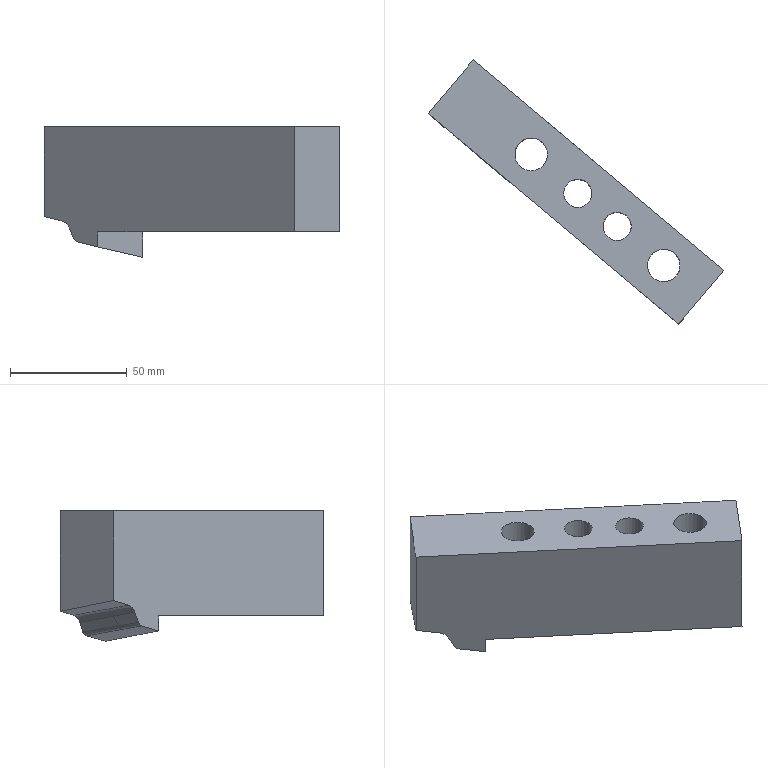Part | NX | features solid 2 | 1 solid | 23 faces | box 126.53 x 112.972 x 55.836 mm | volume 160707 mm3 | plane 9 | spline 8 | cylinder 6 | commonest cylinder face diameters 12 x2 14 x2 20 x2
STEP:
#1=CARTESIAN_POINT('',(-530.147,-22.288,55.));
#2=VERTEX_POINT('',#1);
#3=CARTESIAN_POINT('',(-534.743,-18.432,55.));
#4=DIRECTION('',(0.,0.,1.));
#5=DIRECTION('',(0.766,-0.6428,0.));
#6=AXIS2_PLACEMENT_3D('',#3,#4,#5);
#7=CIRCLE('',#6,6.);
#8=EDGE_CURVE('',#2,#2,#7,.T.);
#9=ORIENTED_EDGE('',*,*,#8,.T.);
#10=EDGE_LOOP('',(#9));
#11=FACE_BOUND('',#10,.T.);
#12=CARTESIAN_POINT('',(-563.853,5.994,55.));
#13=VERTEX_POINT('',#12);
#14=CARTESIAN_POINT('',(-571.513,12.422,55.));
#15=DIRECTION('',(0.,0.,1.));
#16=DIRECTION('',(0.766,-0.6428,0.));
#17=AXIS2_PLACEMENT_3D('',#14,#15,#16);
#18=CIRCLE('',#17,10.);
#19=EDGE_CURVE('',#13,#13,#18,.T.);
#20=ORIENTED_EDGE('',*,*,#19,.T.);
#21=EDGE_LOOP('',(#20));
#22=FACE_BOUND('',#21,.T.);
#23=CARTESIAN_POINT('',(-507.165,-41.572,55.));
#24=VERTEX_POINT('',#23);
#25=CARTESIAN_POINT('',(-514.826,-35.144,55.));
#26=DIRECTION('',(0.,0.,1.));
#27=DIRECTION('',(0.766,-0.6428,0.));
#28=AXIS2_PLACEMENT_3D('',#25,#26,#27);
#29=CIRCLE('',#28,10.);
#30=EDGE_CURVE('',#24,#24,#29,.T.);
#31=ORIENTED_EDGE('',*,*,#30,.T.);
#32=EDGE_LOOP('',(#31));
#33=FACE_BOUND('',#32,.T.);
#34=CARTESIAN_POINT('',(-547.,-8.147,55.));
#35=VERTEX_POINT('',#34);
#36=CARTESIAN_POINT('',(-551.596,-4.29,55.));
#37=DIRECTION('',(0.,0.,1.));
#38=DIRECTION('',(0.766,-0.6428,0.));
#39=AXIS2_PLACEMENT_3D('',#36,#37,#38);
#40=CIRCLE('',#39,6.);
#41=EDGE_CURVE('',#35,#35,#40,.T.);
#42=ORIENTED_EDGE('',*,*,#41,.T.);
#43=EDGE_LOOP('',(#42));
#44=FACE_BOUND('',#43,.T.);
#45=CARTESIAN_POINT('',(-508.381,-60.133,55.));
#46=VERTEX_POINT('',#45);
#47=CARTESIAN_POINT('',(-592.646,10.573,55.));
#48=VERTEX_POINT('',#47);
#49=CARTESIAN_POINT('',(-527.532,-44.064,55.));
#50=DIRECTION('',(0.766,-0.6428,0.));
#51=VECTOR('',#50,1000.);
#52=LINE('',#49,#51);
#53=EDGE_CURVE('',#46,#48,#52,.F.);
#54=ORIENTED_EDGE('',*,*,#53,.T.);
#55=CARTESIAN_POINT('',(-573.362,33.555,55.));
#56=VERTEX_POINT('',#55);
#57=CARTESIAN_POINT('',(-592.646,10.573,55.));
#58=DIRECTION('',(-0.6428,-0.766,0.));
#59=VECTOR('',#58,1000.);
#60=LINE('',#57,#59);
#61=EDGE_CURVE('',#48,#56,#60,.F.);
#62=ORIENTED_EDGE('',*,*,#61,.T.);
#63=CARTESIAN_POINT('',(-489.097,-37.152,55.));
#64=VERTEX_POINT('',#63);
#65=CARTESIAN_POINT('',(-508.248,-21.082,55.));
#66=DIRECTION('',(0.766,-0.6428,0.));
#67=VECTOR('',#66,1000.);
#68=LINE('',#65,#67);
#69=EDGE_CURVE('',#64,#56,#68,.F.);
#70=ORIENTED_EDGE('',*,*,#69,.F.);
#71=CARTESIAN_POINT('',(-534.092,-90.775,55.));
#72=DIRECTION('',(-0.6428,-0.766,0.));
#73=VECTOR('',#72,1000.);
#74=LINE('',#71,#73);
#75=EDGE_CURVE('',#46,#64,#74,.F.);
#76=ORIENTED_EDGE('',*,*,#75,.F.);
#77=EDGE_LOOP('',(#54,#62,#70,#76));
#78=FACE_BOUND('',#77,.T.);
#79=CARTESIAN_POINT('',(-527.532,-44.064,55.));
#80=DIRECTION('',(0.,0.,1.));
#81=DIRECTION('',(0.6428,0.766,0.));
#82=AXIS2_PLACEMENT_3D('',#79,#80,#81);
#83=PLANE('',#82);
#84=ADVANCED_FACE('',(#11,#22,#33,#44,#78),#83,.F.);
#85=CARTESIAN_POINT('',(-615.627,29.857,100.));
#86=VERTEX_POINT('',#85);
#87=CARTESIAN_POINT('',(-596.343,52.838,100.));
#88=VERTEX_POINT('',#87);
#89=CARTESIAN_POINT('',(-567.418,87.31,100.));
#90=DIRECTION('',(0.6428,0.766,0.));
#91=VECTOR('',#90,1000.);
#92=LINE('',#89,#91);
#93=EDGE_CURVE('',#86,#88,#92,.T.);
#94=ORIENTED_EDGE('',*,*,#93,.F.);
#95=CARTESIAN_POINT('',(-508.381,-60.133,100.));
#96=VERTEX_POINT('',#95);
#97=CARTESIAN_POINT('',(-611.797,26.643,100.));
#98=DIRECTION('',(-0.766,0.6428,0.));
#99=VECTOR('',#98,1000.);
#100=LINE('',#97,#99);
#101=EDGE_CURVE('',#96,#86,#100,.T.);
#102=ORIENTED_EDGE('',*,*,#101,.F.);
#103=CARTESIAN_POINT('',(-489.097,-37.152,100.));
#104=VERTEX_POINT('',#103);
#105=CARTESIAN_POINT('',(-460.172,-2.68,100.));
#106=DIRECTION('',(0.6428,0.766,0.));
#107=VECTOR('',#106,1000.);
#108=LINE('',#105,#107);
#109=EDGE_CURVE('',#96,#104,#108,.T.);
#110=ORIENTED_EDGE('',*,*,#109,.T.);
#111=CARTESIAN_POINT('',(-592.513,49.624,100.));
#112=DIRECTION('',(-0.766,0.6428,0.));
#113=VECTOR('',#112,1000.);
#114=LINE('',#111,#113);
#115=EDGE_CURVE('',#104,#88,#114,.T.);
#116=ORIENTED_EDGE('',*,*,#115,.T.);
#117=EDGE_LOOP('',(#94,#102,#110,#116));
#118=FACE_BOUND('',#117,.T.);
#119=CARTESIAN_POINT('',(-534.743,-24.432,100.));
#120=VERTEX_POINT('',#119);
#121=CARTESIAN_POINT('',(-534.743,-18.432,100.));
#122=DIRECTION('',(0.,0.,1.));
#123=DIRECTION('',(0.,-1.,0.));
#124=AXIS2_PLACEMENT_3D('',#121,#122,#123);
#125=CIRCLE('',#124,6.);
#126=EDGE_CURVE('',#120,#120,#125,.T.);
#127=ORIENTED_EDGE('',*,*,#126,.F.);
#128=EDGE_LOOP('',(#127));
#129=FACE_BOUND('',#128,.T.);
#130=CARTESIAN_POINT('',(-514.826,-42.144,100.));
#131=VERTEX_POINT('',#130);
#132=CARTESIAN_POINT('',(-514.826,-35.144,100.));
#133=DIRECTION('',(0.,0.,1.));
#134=DIRECTION('',(0.,-1.,0.));
#135=AXIS2_PLACEMENT_3D('',#132,#133,#134);
#136=CIRCLE('',#135,7.);
#137=EDGE_CURVE('',#131,#131,#136,.T.);
#138=ORIENTED_EDGE('',*,*,#137,.F.);
#139=EDGE_LOOP('',(#138));
#140=FACE_BOUND('',#139,.T.);
#141=CARTESIAN_POINT('',(-571.513,5.422,100.));
#142=VERTEX_POINT('',#141);
#143=CARTESIAN_POINT('',(-571.513,12.422,100.));
#144=DIRECTION('',(0.,0.,1.));
#145=DIRECTION('',(0.,-1.,0.));
#146=AXIS2_PLACEMENT_3D('',#143,#144,#145);
#147=CIRCLE('',#146,7.);
#148=EDGE_CURVE('',#142,#142,#147,.T.);
#149=ORIENTED_EDGE('',*,*,#148,.F.);
#150=EDGE_LOOP('',(#149));
#151=FACE_BOUND('',#150,.T.);
#152=CARTESIAN_POINT('',(-551.596,-10.29,100.));
#153=VERTEX_POINT('',#152);
#154=CARTESIAN_POINT('',(-551.596,-4.29,100.));
#155=DIRECTION('',(0.,0.,1.));
#156=DIRECTION('',(0.,-1.,0.));
#157=AXIS2_PLACEMENT_3D('',#154,#155,#156);
#158=CIRCLE('',#157,6.);
#159=EDGE_CURVE('',#153,#153,#158,.T.);
#160=ORIENTED_EDGE('',*,*,#159,.F.);
#161=EDGE_LOOP('',(#160));
#162=FACE_BOUND('',#161,.T.);
#163=CARTESIAN_POINT('',(-563.588,84.096,100.));
#164=DIRECTION('',(0.,0.,1.));
#165=DIRECTION('',(0.766,-0.6428,0.));
#166=AXIS2_PLACEMENT_3D('',#163,#164,#165);
#167=PLANE('',#166);
#168=ADVANCED_FACE('',(#118,#129,#140,#151,#162),#167,.T.);
#169=CARTESIAN_POINT('',(-508.381,-60.133,75.));
#170=DIRECTION('',(0.,0.,1.));
#171=VECTOR('',#170,1000.);
#172=LINE('',#169,#171);
#173=EDGE_CURVE('',#46,#96,#172,.T.);
#174=ORIENTED_EDGE('',*,*,#173,.F.);
#175=ORIENTED_EDGE('',*,*,#75,.T.);
#176=CARTESIAN_POINT('',(-489.097,-37.152,75.));
#177=DIRECTION('',(0.,0.,1.));
#178=VECTOR('',#177,1000.);
#179=LINE('',#176,#178);
#180=EDGE_CURVE('',#64,#104,#179,.T.);
#181=ORIENTED_EDGE('',*,*,#180,.T.);
#182=ORIENTED_EDGE('',*,*,#109,.F.);
#183=EDGE_LOOP('',(#174,#175,#181,#182));
#184=FACE_BOUND('',#183,.T.);
#185=CARTESIAN_POINT('',(-534.092,-90.775,75.));
#186=DIRECTION('',(0.766,-0.6428,0.));
#187=DIRECTION('',(0.,0.,-1.));
#188=AXIS2_PLACEMENT_3D('',#185,#186,#187);
#189=PLANE('',#188);
#190=ADVANCED_FACE('',(#184),#189,.T.);
#191=CARTESIAN_POINT('',(-615.627,29.857,61.582));
#192=VERTEX_POINT('',#191);
#193=CARTESIAN_POINT('',(-615.627,29.857,75.));
#194=DIRECTION('',(0.,0.,-1.));
#195=VECTOR('',#194,1000.);
#196=LINE('',#193,#195);
#197=EDGE_CURVE('',#86,#192,#196,.T.);
#198=ORIENTED_EDGE('',*,*,#197,.T.);
#199=CARTESIAN_POINT('',(-607.971,23.433,59.662));
#200=VERTEX_POINT('',#199);
#201=CARTESIAN_POINT('',(-615.627,29.857,61.582));
#202=CARTESIAN_POINT('',(-613.073,27.714,60.938));
#203=CARTESIAN_POINT('',(-610.518,25.57,60.298));
#204=CARTESIAN_POINT('',(-607.963,23.426,59.66));
#205=B_SPLINE_CURVE_WITH_KNOTS('',3,(#201,#202,#203,#204),.UNSPECIFIED.,.F.,.F.,(4,4),(0.,0.01019),.UNSPECIFIED.);
#206=EDGE_CURVE('',#192,#200,#205,.T.);
#207=ORIENTED_EDGE('',*,*,#206,.T.);
#208=CARTESIAN_POINT('',(-604.808,20.779,56.617));
#209=VERTEX_POINT('',#208);
#210=CARTESIAN_POINT('',(-607.974,23.435,59.663));
#211=CARTESIAN_POINT('',(-606.633,22.31,59.328));
#212=CARTESIAN_POINT('',(-605.455,21.322,58.191));
#213=CARTESIAN_POINT('',(-604.81,20.78,56.621));
#214=B_SPLINE_CURVE_WITH_KNOTS('',3,(#210,#211,#212,#213),.UNSPECIFIED.,.F.,.F.,(4,4),(0.,0.005307),.UNSPECIFIED.);
#215=EDGE_CURVE('',#200,#209,#214,.T.);
#216=ORIENTED_EDGE('',*,*,#215,.T.);
#217=CARTESIAN_POINT('',(-603.017,19.276,52.254));
#218=VERTEX_POINT('',#217);
#219=CARTESIAN_POINT('',(-604.806,20.777,56.612));
#220=CARTESIAN_POINT('',(-604.209,20.276,55.159));
#221=CARTESIAN_POINT('',(-603.612,19.775,53.706));
#222=CARTESIAN_POINT('',(-603.016,19.275,52.252));
#223=B_SPLINE_CURVE_WITH_KNOTS('',3,(#219,#220,#221,#222),.UNSPECIFIED.,.F.,.F.,(4,4),(0.0004927,0.005439),.UNSPECIFIED.);
#224=EDGE_CURVE('',#209,#218,#223,.T.);
#225=ORIENTED_EDGE('',*,*,#224,.T.);
#226=CARTESIAN_POINT('',(-601.43,17.944,50.734));
#227=VERTEX_POINT('',#226);
#228=CARTESIAN_POINT('',(-603.018,19.277,52.257));
#229=CARTESIAN_POINT('',(-602.695,19.006,51.469));
#230=CARTESIAN_POINT('',(-602.103,18.509,50.899));
#231=CARTESIAN_POINT('',(-601.431,17.945,50.734));
#232=B_SPLINE_CURVE_WITH_KNOTS('',3,(#228,#229,#230,#231),.UNSPECIFIED.,.F.,.F.,(4,4),(0.,0.002661),.UNSPECIFIED.);
#233=EDGE_CURVE('',#218,#227,#232,.T.);
#234=ORIENTED_EDGE('',*,*,#233,.T.);
#235=CARTESIAN_POINT('',(-592.646,10.573,48.586));
#236=VERTEX_POINT('',#235);
#237=CARTESIAN_POINT('',(-601.426,17.941,50.733));
#238=CARTESIAN_POINT('',(-598.5,15.486,50.012));
#239=CARTESIAN_POINT('',(-595.573,13.03,49.297));
#240=CARTESIAN_POINT('',(-592.646,10.573,48.586));
#241=B_SPLINE_CURVE_WITH_KNOTS('',3,(#237,#238,#239,#240),.UNSPECIFIED.,.F.,.F.,(4,4),(0.01887,0.03053),.UNSPECIFIED.);
#242=EDGE_CURVE('',#227,#236,#241,.T.);
#243=ORIENTED_EDGE('',*,*,#242,.T.);
#244=CARTESIAN_POINT('',(-592.646,10.573,105.));
#245=DIRECTION('',(0.,0.,1.));
#246=VECTOR('',#245,1000.);
#247=LINE('',#244,#246);
#248=EDGE_CURVE('',#48,#236,#247,.F.);
#249=ORIENTED_EDGE('',*,*,#248,.F.);
#250=ORIENTED_EDGE('',*,*,#53,.F.);
#251=ORIENTED_EDGE('',*,*,#173,.T.);
#252=ORIENTED_EDGE('',*,*,#101,.T.);
#253=EDGE_LOOP('',(#198,#207,#216,#225,#234,#243,#249,#250,#251,#252));
#254=FACE_BOUND('',#253,.T.);
#255=CARTESIAN_POINT('',(-550.513,-24.78,75.));
#256=DIRECTION('',(0.6428,0.766,0.));
#257=DIRECTION('',(0.,0.,1.));
#258=AXIS2_PLACEMENT_3D('',#255,#256,#257);
#259=PLANE('',#258);
#260=ADVANCED_FACE('',(#254),#259,.F.);
#261=CARTESIAN_POINT('',(-596.343,52.838,56.979));
#262=VERTEX_POINT('',#261);
#263=CARTESIAN_POINT('',(-589.544,47.133,55.322));
#264=VERTEX_POINT('',#263);
#265=CARTESIAN_POINT('',(-596.343,52.838,56.979));
#266=CARTESIAN_POINT('',(-594.077,50.936,56.424));
#267=CARTESIAN_POINT('',(-591.81,49.034,55.871));
#268=CARTESIAN_POINT('',(-589.542,47.131,55.322));
#269=B_SPLINE_CURVE_WITH_KNOTS('',3,(#265,#266,#267,#268),.UNSPECIFIED.,.F.,.F.,(4,4),(0.,0.009031),.UNSPECIFIED.);
#270=EDGE_CURVE('',#262,#264,#269,.T.);
#271=ORIENTED_EDGE('',*,*,#270,.F.);
#272=CARTESIAN_POINT('',(-596.343,52.838,-200.));
#273=DIRECTION('',(0.,0.,-1.));
#274=VECTOR('',#273,1000.);
#275=LINE('',#272,#274);
#276=EDGE_CURVE('',#88,#262,#275,.T.);
#277=ORIENTED_EDGE('',*,*,#276,.F.);
#278=ORIENTED_EDGE('',*,*,#115,.F.);
#279=ORIENTED_EDGE('',*,*,#180,.F.);
#280=ORIENTED_EDGE('',*,*,#69,.T.);
#281=CARTESIAN_POINT('',(-573.362,33.555,44.164));
#282=VERTEX_POINT('',#281);
#283=CARTESIAN_POINT('',(-573.362,33.555,105.));
#284=DIRECTION('',(0.,0.,1.));
#285=VECTOR('',#284,1000.);
#286=LINE('',#283,#285);
#287=EDGE_CURVE('',#56,#282,#286,.F.);
#288=ORIENTED_EDGE('',*,*,#287,.T.);
#289=CARTESIAN_POINT('',(-583.064,41.696,46.466));
#290=VERTEX_POINT('',#289);
#291=CARTESIAN_POINT('',(-583.068,41.699,46.467));
#292=CARTESIAN_POINT('',(-579.834,38.985,45.694));
#293=CARTESIAN_POINT('',(-576.598,36.27,44.926));
#294=CARTESIAN_POINT('',(-573.362,33.555,44.164));
#295=B_SPLINE_CURVE_WITH_KNOTS('',3,(#291,#292,#293,#294),.UNSPECIFIED.,.F.,.F.,(4,4),(0.01762,0.0305),.UNSPECIFIED.);
#296=EDGE_CURVE('',#290,#282,#295,.T.);
#297=ORIENTED_EDGE('',*,*,#296,.F.);
#298=CARTESIAN_POINT('',(-584.684,43.055,48.042));
#299=VERTEX_POINT('',#298);
#300=CARTESIAN_POINT('',(-584.683,43.054,48.04));
#301=CARTESIAN_POINT('',(-584.362,42.784,47.224));
#302=CARTESIAN_POINT('',(-583.754,42.275,46.631));
#303=CARTESIAN_POINT('',(-583.063,41.694,46.466));
#304=B_SPLINE_CURVE_WITH_KNOTS('',3,(#300,#301,#302,#303),.UNSPECIFIED.,.F.,.F.,(4,4),(0.,0.002732),.UNSPECIFIED.);
#305=EDGE_CURVE('',#299,#290,#304,.T.);
#306=ORIENTED_EDGE('',*,*,#305,.F.);
#307=CARTESIAN_POINT('',(-586.313,44.422,52.174));
#308=VERTEX_POINT('',#307);
#309=CARTESIAN_POINT('',(-586.312,44.421,52.171));
#310=CARTESIAN_POINT('',(-585.77,43.966,50.796));
#311=CARTESIAN_POINT('',(-585.227,43.511,49.42));
#312=CARTESIAN_POINT('',(-584.685,43.055,48.044));
#313=B_SPLINE_CURVE_WITH_KNOTS('',3,(#309,#310,#311,#312),.UNSPECIFIED.,.F.,.F.,(4,4),(0.00009556,0.004737),.UNSPECIFIED.);
#314=EDGE_CURVE('',#308,#299,#313,.T.);
#315=ORIENTED_EDGE('',*,*,#314,.F.);
#316=CARTESIAN_POINT('',(-589.545,47.134,55.322));
#317=CARTESIAN_POINT('',(-588.166,45.977,54.988));
#318=CARTESIAN_POINT('',(-586.956,44.961,53.804));
#319=CARTESIAN_POINT('',(-586.314,44.423,52.176));
#320=B_SPLINE_CURVE_WITH_KNOTS('',3,(#316,#317,#318,#319),.UNSPECIFIED.,.F.,.F.,(4,4),(0.,0.005448),.UNSPECIFIED.);
#321=EDGE_CURVE('',#264,#308,#320,.T.);
#322=ORIENTED_EDGE('',*,*,#321,.F.);
#323=EDGE_LOOP('',(#271,#277,#278,#279,#280,#288,#297,#306,#315,#322));
#324=FACE_BOUND('',#323,.T.);
#325=CARTESIAN_POINT('',(-531.23,-1.799,-200.));
#326=DIRECTION('',(0.6428,0.766,0.));
#327=DIRECTION('',(0.,0.,1.));
#328=AXIS2_PLACEMENT_3D('',#325,#326,#327);
#329=PLANE('',#328);
#330=ADVANCED_FACE('',(#324),#329,.T.);
#331=CARTESIAN_POINT('',(-507.165,-41.572,75.));
#332=VERTEX_POINT('',#331);
#333=CARTESIAN_POINT('',(-514.826,-35.144,75.));
#334=DIRECTION('',(0.,0.,1.));
#335=DIRECTION('',(0.766,-0.6428,0.));
#336=AXIS2_PLACEMENT_3D('',#333,#334,#335);
#337=CIRCLE('',#336,10.);
#338=EDGE_CURVE('',#332,#332,#337,.F.);
#339=ORIENTED_EDGE('',*,*,#338,.F.);
#340=EDGE_LOOP('',(#339));
#341=FACE_BOUND('',#340,.T.);
#342=ORIENTED_EDGE('',*,*,#30,.F.);
#343=EDGE_LOOP('',(#342));
#344=FACE_BOUND('',#343,.T.);
#345=CARTESIAN_POINT('',(-514.826,-35.144,72.));
#346=DIRECTION('',(0.,0.,-1.));
#347=DIRECTION('',(0.766,-0.6428,0.));
#348=AXIS2_PLACEMENT_3D('',#345,#346,#347);
#349=CYLINDRICAL_SURFACE('',#348,10.);
#350=ADVANCED_FACE('',(#341,#344),#349,.F.);
#351=CARTESIAN_POINT('',(-563.853,5.994,75.));
#352=VERTEX_POINT('',#351);
#353=CARTESIAN_POINT('',(-571.513,12.422,75.));
#354=DIRECTION('',(0.,0.,-1.));
#355=DIRECTION('',(0.766,-0.6428,0.));
#356=AXIS2_PLACEMENT_3D('',#353,#354,#355);
#357=CIRCLE('',#356,10.);
#358=EDGE_CURVE('',#352,#352,#357,.T.);
#359=ORIENTED_EDGE('',*,*,#358,.F.);
#360=EDGE_LOOP('',(#359));
#361=FACE_BOUND('',#360,.T.);
#362=ORIENTED_EDGE('',*,*,#19,.F.);
#363=EDGE_LOOP('',(#362));
#364=FACE_BOUND('',#363,.T.);
#365=CARTESIAN_POINT('',(-571.513,12.422,75.));
#366=DIRECTION('',(0.,0.,-1.));
#367=DIRECTION('',(0.766,-0.6428,0.));
#368=AXIS2_PLACEMENT_3D('',#365,#366,#367);
#369=CYLINDRICAL_SURFACE('',#368,10.);
#370=ADVANCED_FACE('',(#361,#364),#369,.F.);
#371=CARTESIAN_POINT('',(-509.464,-39.644,75.));
#372=VERTEX_POINT('',#371);
#373=CARTESIAN_POINT('',(-514.826,-35.144,75.));
#374=DIRECTION('',(0.,0.,1.));
#375=DIRECTION('',(0.766,-0.6428,0.));
#376=AXIS2_PLACEMENT_3D('',#373,#374,#375);
#377=CIRCLE('',#376,7.);
#378=EDGE_CURVE('',#372,#372,#377,.T.);
#379=ORIENTED_EDGE('',*,*,#378,.T.);
#380=EDGE_LOOP('',(#379));
#381=FACE_BOUND('',#380,.T.);
#382=ORIENTED_EDGE('',*,*,#338,.T.);
#383=EDGE_LOOP('',(#382));
#384=FACE_BOUND('',#383,.T.);
#385=CARTESIAN_POINT('',(-514.826,-35.144,75.));
#386=DIRECTION('',(0.,0.,1.));
#387=DIRECTION('',(-0.766,0.6428,0.));
#388=AXIS2_PLACEMENT_3D('',#385,#386,#387);
#389=PLANE('',#388);
#390=ADVANCED_FACE('',(#381,#384),#389,.F.);
#391=ORIENTED_EDGE('',*,*,#137,.T.);
#392=EDGE_LOOP('',(#391));
#393=FACE_BOUND('',#392,.T.);
#394=ORIENTED_EDGE('',*,*,#378,.F.);
#395=EDGE_LOOP('',(#394));
#396=FACE_BOUND('',#395,.T.);
#397=CARTESIAN_POINT('',(-514.826,-35.144,72.));
#398=DIRECTION('',(0.,0.,1.));
#399=DIRECTION('',(-0.766,0.6428,0.));
#400=AXIS2_PLACEMENT_3D('',#397,#398,#399);
#401=CYLINDRICAL_SURFACE('',#400,7.);
#402=ADVANCED_FACE('',(#393,#396),#401,.F.);
#403=CARTESIAN_POINT('',(-566.151,7.923,75.));
#404=VERTEX_POINT('',#403);
#405=CARTESIAN_POINT('',(-571.513,12.422,75.));
#406=DIRECTION('',(0.,0.,1.));
#407=DIRECTION('',(0.766,-0.6428,0.));
#408=AXIS2_PLACEMENT_3D('',#405,#406,#407);
#409=CIRCLE('',#408,7.);
#410=EDGE_CURVE('',#404,#404,#409,.T.);
#411=ORIENTED_EDGE('',*,*,#410,.T.);
#412=EDGE_LOOP('',(#411));
#413=FACE_BOUND('',#412,.T.);
#414=ORIENTED_EDGE('',*,*,#358,.T.);
#415=EDGE_LOOP('',(#414));
#416=FACE_BOUND('',#415,.T.);
#417=CARTESIAN_POINT('',(-571.513,12.422,75.));
#418=DIRECTION('',(0.,0.,1.));
#419=DIRECTION('',(-0.766,0.6428,0.));
#420=AXIS2_PLACEMENT_3D('',#417,#418,#419);
#421=PLANE('',#420);
#422=ADVANCED_FACE('',(#413,#416),#421,.F.);
#423=ORIENTED_EDGE('',*,*,#148,.T.);
#424=EDGE_LOOP('',(#423));
#425=FACE_BOUND('',#424,.T.);
#426=ORIENTED_EDGE('',*,*,#410,.F.);
#427=EDGE_LOOP('',(#426));
#428=FACE_BOUND('',#427,.T.);
#429=CARTESIAN_POINT('',(-571.513,12.422,75.));
#430=DIRECTION('',(0.,0.,1.));
#431=DIRECTION('',(-0.766,0.6428,0.));
#432=AXIS2_PLACEMENT_3D('',#429,#430,#431);
#433=CYLINDRICAL_SURFACE('',#432,7.);
#434=ADVANCED_FACE('',(#425,#428),#433,.F.);
#435=ORIENTED_EDGE('',*,*,#159,.T.);
#436=EDGE_LOOP('',(#435));
#437=FACE_BOUND('',#436,.T.);
#438=ORIENTED_EDGE('',*,*,#41,.F.);
#439=EDGE_LOOP('',(#438));
#440=FACE_BOUND('',#439,.T.);
#441=CARTESIAN_POINT('',(-551.596,-4.29,105.));
#442=DIRECTION('',(0.,0.,-1.));
#443=DIRECTION('',(-0.766,0.6428,0.));
#444=AXIS2_PLACEMENT_3D('',#441,#442,#443);
#445=CYLINDRICAL_SURFACE('',#444,6.);
#446=ADVANCED_FACE('',(#437,#440),#445,.F.);
#447=ORIENTED_EDGE('',*,*,#126,.T.);
#448=EDGE_LOOP('',(#447));
#449=FACE_BOUND('',#448,.T.);
#450=ORIENTED_EDGE('',*,*,#8,.F.);
#451=EDGE_LOOP('',(#450));
#452=FACE_BOUND('',#451,.T.);
#453=CARTESIAN_POINT('',(-534.743,-18.432,105.));
#454=DIRECTION('',(0.,0.,-1.));
#455=DIRECTION('',(-0.766,0.6428,0.));
#456=AXIS2_PLACEMENT_3D('',#453,#454,#455);
#457=CYLINDRICAL_SURFACE('',#456,6.);
#458=ADVANCED_FACE('',(#449,#452),#457,.F.);
#459=ORIENTED_EDGE('',*,*,#276,.T.);
#460=CARTESIAN_POINT('',(-596.343,52.838,56.979));
#461=CARTESIAN_POINT('',(-602.774,45.175,58.49));
#462=CARTESIAN_POINT('',(-609.201,37.515,60.025));
#463=CARTESIAN_POINT('',(-615.627,29.857,61.582));
#464=B_SPLINE_CURVE_WITH_KNOTS('',3,(#460,#461,#462,#463),.UNSPECIFIED.,.F.,.F.,(4,4),(0.,0.03035),.UNSPECIFIED.);
#465=EDGE_CURVE('',#262,#192,#464,.T.);
#466=ORIENTED_EDGE('',*,*,#465,.T.);
#467=ORIENTED_EDGE('',*,*,#197,.F.);
#468=ORIENTED_EDGE('',*,*,#93,.T.);
#469=EDGE_LOOP('',(#459,#466,#467,#468));
#470=FACE_BOUND('',#469,.T.);
#471=CARTESIAN_POINT('',(-605.985,41.348,80.));
#472=DIRECTION('',(0.766,-0.6428,0.));
#473=DIRECTION('',(0.6428,0.766,0.));
#474=AXIS2_PLACEMENT_3D('',#471,#472,#473);
#475=PLANE('',#474);
#476=ADVANCED_FACE('',(#470),#475,.F.);
#477=ORIENTED_EDGE('',*,*,#248,.T.);
#478=CARTESIAN_POINT('',(-592.646,10.573,48.586));
#479=CARTESIAN_POINT('',(-586.22,18.231,47.089));
#480=CARTESIAN_POINT('',(-579.792,25.892,45.615));
#481=CARTESIAN_POINT('',(-573.362,33.555,44.164));
#482=B_SPLINE_CURVE_WITH_KNOTS('',3,(#478,#479,#480,#481),.UNSPECIFIED.,.F.,.F.,(4,4),(0.,0.03032),.UNSPECIFIED.);
#483=EDGE_CURVE('',#236,#282,#482,.T.);
#484=ORIENTED_EDGE('',*,*,#483,.T.);
#485=ORIENTED_EDGE('',*,*,#287,.F.);
#486=ORIENTED_EDGE('',*,*,#61,.F.);
#487=EDGE_LOOP('',(#477,#484,#485,#486));
#488=FACE_BOUND('',#487,.T.);
#489=CARTESIAN_POINT('',(-592.646,10.573,105.));
#490=DIRECTION('',(-0.766,0.6428,0.));
#491=DIRECTION('',(-0.6428,-0.766,0.));
#492=AXIS2_PLACEMENT_3D('',#489,#490,#491);
#493=PLANE('',#492);
#494=ADVANCED_FACE('',(#488),#493,.F.);
#495=CARTESIAN_POINT('',(-600.786,32.74,57.955));
#496=VERTEX_POINT('',#495);
#497=CARTESIAN_POINT('',(-600.787,32.74,57.955));
#498=CARTESIAN_POINT('',(-601.282,32.103,58.072));
#499=CARTESIAN_POINT('',(-602.499,30.537,58.36));
#500=CARTESIAN_POINT('',(-604.982,27.333,58.949));
#501=CARTESIAN_POINT('',(-606.786,25.009,59.379));
#502=CARTESIAN_POINT('',(-607.974,23.435,59.663));
#503=B_SPLINE_CURVE_WITH_KNOTS('',3,(#497,#498,#499,#500,#501,#502),.UNSPECIFIED.,.F.,.F.,(4,1,1,4),(0.,0.02406,0.04812,0.09624),.UNSPECIFIED.);
#504=EDGE_CURVE('',#496,#200,#503,.T.);
#505=ORIENTED_EDGE('',*,*,#504,.F.);
#506=CARTESIAN_POINT('',(-597.767,29.822,54.892));
#507=VERTEX_POINT('',#506);
#508=CARTESIAN_POINT('',(-597.767,29.822,54.892));
#509=CARTESIAN_POINT('',(-598.286,30.515,56.461));
#510=CARTESIAN_POINT('',(-599.429,31.62,57.62));
#511=CARTESIAN_POINT('',(-600.787,32.74,57.955));
#512=B_SPLINE_CURVE_WITH_KNOTS('',3,(#508,#509,#510,#511),.UNSPECIFIED.,.F.,.F.,(4,4),(0.,1.),.UNSPECIFIED.);
#513=EDGE_CURVE('',#507,#496,#512,.T.);
#514=ORIENTED_EDGE('',*,*,#513,.F.);
#515=CARTESIAN_POINT('',(-604.81,20.781,56.621));
#516=CARTESIAN_POINT('',(-603.664,22.281,56.336));
#517=CARTESIAN_POINT('',(-601.887,24.544,55.889));
#518=CARTESIAN_POINT('',(-599.445,27.675,55.296));
#519=CARTESIAN_POINT('',(-598.253,29.2,55.009));
#520=CARTESIAN_POINT('',(-597.767,29.822,54.892));
#521=B_SPLINE_CURVE_WITH_KNOTS('',3,(#515,#516,#517,#518,#519,#520),.UNSPECIFIED.,.F.,.F.,(4,1,1,4),(0.9056,0.9528,0.9764,1.),.UNSPECIFIED.);
#522=EDGE_CURVE('',#209,#507,#521,.T.);
#523=ORIENTED_EDGE('',*,*,#522,.F.);
#524=ORIENTED_EDGE('',*,*,#215,.F.);
#525=EDGE_LOOP('',(#505,#514,#523,#524));
#526=FACE_BOUND('',#525,.T.);
#527=CARTESIAN_POINT('',(-604.996,20.537,56.668));
#528=CARTESIAN_POINT('',(-605.317,20.946,57.589));
#529=CARTESIAN_POINT('',(-605.811,21.466,58.402));
#530=CARTESIAN_POINT('',(-606.458,22.071,59.044));
#531=CARTESIAN_POINT('',(-607.213,22.719,59.473));
#532=CARTESIAN_POINT('',(-608.024,23.368,59.675));
#533=CARTESIAN_POINT('',(-604.742,20.871,56.604));
#534=CARTESIAN_POINT('',(-605.061,21.281,57.527));
#535=CARTESIAN_POINT('',(-605.555,21.802,58.34));
#536=CARTESIAN_POINT('',(-606.201,22.409,58.982));
#537=CARTESIAN_POINT('',(-606.955,23.06,59.411));
#538=CARTESIAN_POINT('',(-607.765,23.712,59.613));
#539=CARTESIAN_POINT('',(-604.487,21.203,56.541));
#540=CARTESIAN_POINT('',(-604.805,21.615,57.464));
#541=CARTESIAN_POINT('',(-605.298,22.138,58.277));
#542=CARTESIAN_POINT('',(-605.943,22.747,58.921));
#543=CARTESIAN_POINT('',(-606.697,23.399,59.349));
#544=CARTESIAN_POINT('',(-607.506,24.053,59.551));
#545=CARTESIAN_POINT('',(-604.23,21.536,56.477));
#546=CARTESIAN_POINT('',(-604.548,21.949,57.401));
#547=CARTESIAN_POINT('',(-605.039,22.473,58.215));
#548=CARTESIAN_POINT('',(-605.684,23.084,58.859));
#549=CARTESIAN_POINT('',(-606.437,23.739,59.288));
#550=CARTESIAN_POINT('',(-607.246,24.394,59.489));
#551=CARTESIAN_POINT('',(-603.691,22.233,56.342));
#552=CARTESIAN_POINT('',(-604.007,22.647,57.268));
#553=CARTESIAN_POINT('',(-604.497,23.174,58.083));
#554=CARTESIAN_POINT('',(-605.141,23.788,58.728));
#555=CARTESIAN_POINT('',(-605.893,24.446,59.158));
#556=CARTESIAN_POINT('',(-606.701,25.106,59.359));
#557=CARTESIAN_POINT('',(-603.139,22.942,56.204));
#558=CARTESIAN_POINT('',(-603.454,23.357,57.132));
#559=CARTESIAN_POINT('',(-603.943,23.885,57.949));
#560=CARTESIAN_POINT('',(-604.587,24.502,58.596));
#561=CARTESIAN_POINT('',(-605.339,25.163,59.026));
#562=CARTESIAN_POINT('',(-606.148,25.824,59.227));
#563=CARTESIAN_POINT('',(-602.885,23.268,56.14));
#564=CARTESIAN_POINT('',(-603.199,23.682,57.069));
#565=CARTESIAN_POINT('',(-603.689,24.212,57.888));
#566=CARTESIAN_POINT('',(-604.332,24.829,58.535));
#567=CARTESIAN_POINT('',(-605.085,25.49,58.966));
#568=CARTESIAN_POINT('',(-605.894,26.153,59.166));
#569=CARTESIAN_POINT('',(-602.275,24.049,55.988));
#570=CARTESIAN_POINT('',(-602.589,24.464,56.92));
#571=CARTESIAN_POINT('',(-603.078,24.995,57.74));
#572=CARTESIAN_POINT('',(-603.722,25.613,58.389));
#573=CARTESIAN_POINT('',(-604.475,26.277,58.82));
#574=CARTESIAN_POINT('',(-605.285,26.942,59.021));
#575=CARTESIAN_POINT('',(-601.664,24.831,55.838));
#576=CARTESIAN_POINT('',(-601.978,25.247,56.771));
#577=CARTESIAN_POINT('',(-602.466,25.778,57.593));
#578=CARTESIAN_POINT('',(-603.111,26.398,58.244));
#579=CARTESIAN_POINT('',(-603.865,27.063,58.676));
#580=CARTESIAN_POINT('',(-604.676,27.729,58.877));
#581=CARTESIAN_POINT('',(-601.343,25.243,55.759));
#582=CARTESIAN_POINT('',(-601.656,25.658,56.693));
#583=CARTESIAN_POINT('',(-602.145,26.189,57.516));
#584=CARTESIAN_POINT('',(-602.79,26.81,58.167));
#585=CARTESIAN_POINT('',(-603.544,27.475,58.599));
#586=CARTESIAN_POINT('',(-604.356,28.142,58.8));
#587=CARTESIAN_POINT('',(-600.701,26.065,55.601));
#588=CARTESIAN_POINT('',(-601.013,26.481,56.537));
#589=CARTESIAN_POINT('',(-601.502,27.013,57.362));
#590=CARTESIAN_POINT('',(-602.147,27.634,58.014));
#591=CARTESIAN_POINT('',(-602.903,28.301,58.447));
#592=CARTESIAN_POINT('',(-603.715,28.969,58.648));
#593=CARTESIAN_POINT('',(-600.059,26.888,55.445));
#594=CARTESIAN_POINT('',(-600.371,27.304,56.382));
#595=CARTESIAN_POINT('',(-600.86,27.836,57.209));
#596=CARTESIAN_POINT('',(-601.505,28.458,57.862));
#597=CARTESIAN_POINT('',(-602.261,29.126,58.295));
#598=CARTESIAN_POINT('',(-603.074,29.795,58.496));
#599=CARTESIAN_POINT('',(-599.737,27.3,55.367));
#600=CARTESIAN_POINT('',(-600.049,27.715,56.305));
#601=CARTESIAN_POINT('',(-600.538,28.248,57.132));
#602=CARTESIAN_POINT('',(-601.184,28.871,57.785));
#603=CARTESIAN_POINT('',(-601.94,29.539,58.219));
#604=CARTESIAN_POINT('',(-602.754,30.208,58.42));
#605=CARTESIAN_POINT('',(-599.124,28.085,55.219));
#606=CARTESIAN_POINT('',(-599.436,28.501,56.158));
#607=CARTESIAN_POINT('',(-599.925,29.034,56.986));
#608=CARTESIAN_POINT('',(-600.571,29.657,57.64));
#609=CARTESIAN_POINT('',(-601.328,30.327,58.074));
#610=CARTESIAN_POINT('',(-602.141,30.997,58.275));
#611=CARTESIAN_POINT('',(-598.51,28.871,55.071));
#612=CARTESIAN_POINT('',(-598.822,29.286,56.011));
#613=CARTESIAN_POINT('',(-599.311,29.82,56.84));
#614=CARTESIAN_POINT('',(-599.957,30.444,57.495));
#615=CARTESIAN_POINT('',(-600.715,31.114,57.929));
#616=CARTESIAN_POINT('',(-601.529,31.785,58.13));
#617=CARTESIAN_POINT('',(-598.245,29.21,55.007));
#618=CARTESIAN_POINT('',(-598.557,29.626,55.947));
#619=CARTESIAN_POINT('',(-599.046,30.16,56.777));
#620=CARTESIAN_POINT('',(-599.692,30.784,57.432));
#621=CARTESIAN_POINT('',(-600.45,31.454,57.867));
#622=CARTESIAN_POINT('',(-601.264,32.126,58.068));
#623=CARTESIAN_POINT('',(-598.001,29.522,54.948));
#624=CARTESIAN_POINT('',(-598.313,29.938,55.889));
#625=CARTESIAN_POINT('',(-598.802,30.472,56.719));
#626=CARTESIAN_POINT('',(-599.448,31.097,57.374));
#627=CARTESIAN_POINT('',(-600.206,31.767,57.809));
#628=CARTESIAN_POINT('',(-601.021,32.439,58.01));
#629=CARTESIAN_POINT('',(-597.767,29.822,54.892));
#630=CARTESIAN_POINT('',(-598.078,30.238,55.833));
#631=CARTESIAN_POINT('',(-598.567,30.772,56.663));
#632=CARTESIAN_POINT('',(-599.214,31.397,57.319));
#633=CARTESIAN_POINT('',(-599.972,32.068,57.754));
#634=CARTESIAN_POINT('',(-600.787,32.74,57.955));
#635=B_SPLINE_SURFACE_WITH_KNOTS('',5,5,((#527,#528,#529,#530,#531,#532),(#533,#534,#535,#536,#537,#538),(#539,#540,#541,#542,#543,#544),(#545,#546,#547,#548,#549,#550),(#551,#552,#553,#554,#555,#556),(#557,#558,#559,#560,#561,#562),(#563,#564,#565,#566,#567,#568),(#569,#570,#571,#572,#573,#574),(#575,#576,#577,#578,#579,#580),(#581,#582,#583,#584,#585,#586),(#587,#588,#589,#590,#591,#592),(#593,#594,#595,#596,#597,#598),(#599,#600,#601,#602,#603,#604),(#605,#606,#607,#608,#609,#610),(#611,#612,#613,#614,#615,#616),(#617,#618,#619,#620,#621,#622),(#623,#624,#625,#626,#627,#628),(#629,#630,#631,#632,#633,#634)),.UNSPECIFIED.,.F.,.F.,.F.,(6,3,3,3,3,6),(6,6),(0.9031,0.9206,0.9394,0.9602,0.981,1.),(0.,1.),.UNSPECIFIED.);
#636=ADVANCED_FACE('',(#526),#635,.F.);
#637=ORIENTED_EDGE('',*,*,#522,.T.);
#638=CARTESIAN_POINT('',(-596.377,27.999,50.726));
#639=VERTEX_POINT('',#638);
#640=CARTESIAN_POINT('',(-596.378,27.998,50.726));
#641=CARTESIAN_POINT('',(-596.841,28.606,52.115));
#642=CARTESIAN_POINT('',(-597.304,29.214,53.503));
#643=CARTESIAN_POINT('',(-597.767,29.822,54.892));
#644=B_SPLINE_CURVE_WITH_KNOTS('',3,(#640,#641,#642,#643),.UNSPECIFIED.,.F.,.F.,(4,4),(0.,1.),.UNSPECIFIED.);
#645=EDGE_CURVE('',#639,#507,#644,.T.);
#646=ORIENTED_EDGE('',*,*,#645,.F.);
#647=CARTESIAN_POINT('',(-603.016,19.275,52.252));
#648=CARTESIAN_POINT('',(-601.982,20.663,52.011));
#649=CARTESIAN_POINT('',(-599.738,23.625,51.492));
#650=CARTESIAN_POINT('',(-597.501,26.538,50.981));
#651=CARTESIAN_POINT('',(-596.378,27.998,50.726));
#652=B_SPLINE_CURVE_WITH_KNOTS('',3,(#647,#648,#649,#650,#651),.UNSPECIFIED.,.F.,.F.,(4,1,4),(0.9099,0.955,1.),.UNSPECIFIED.);
#653=EDGE_CURVE('',#218,#639,#652,.T.);
#654=ORIENTED_EDGE('',*,*,#653,.F.);
#655=ORIENTED_EDGE('',*,*,#224,.F.);
#656=EDGE_LOOP('',(#637,#646,#654,#655));
#657=FACE_BOUND('',#656,.T.);
#658=CARTESIAN_POINT('',(-597.796,29.86,54.979));
#659=CARTESIAN_POINT('',(-596.356,27.97,50.662));
#660=CARTESIAN_POINT('',(-598.784,28.591,55.211));
#661=CARTESIAN_POINT('',(-597.331,26.709,50.89));
#662=CARTESIAN_POINT('',(-599.772,27.321,55.444));
#663=CARTESIAN_POINT('',(-598.305,25.447,51.118));
#664=CARTESIAN_POINT('',(-600.758,26.05,55.677));
#665=CARTESIAN_POINT('',(-599.277,24.184,51.347));
#666=CARTESIAN_POINT('',(-602.188,24.209,56.015));
#667=CARTESIAN_POINT('',(-600.68,22.351,51.677));
#668=CARTESIAN_POINT('',(-603.613,22.363,56.352));
#669=CARTESIAN_POINT('',(-602.072,20.511,52.005));
#670=CARTESIAN_POINT('',(-604.035,21.814,56.452));
#671=CARTESIAN_POINT('',(-602.484,19.964,52.103));
#672=CARTESIAN_POINT('',(-604.446,21.276,56.55));
#673=CARTESIAN_POINT('',(-602.885,19.428,52.198));
#674=CARTESIAN_POINT('',(-604.855,20.736,56.647));
#675=CARTESIAN_POINT('',(-603.286,18.89,52.292));
#676=B_SPLINE_SURFACE_WITH_KNOTS('',5,1,((#658,#659),(#660,#661),(#662,#663),(#664,#665),(#666,#667),(#668,#669),(#670,#671),(#672,#673),(#674,#675)),.RULED_SURF.,.F.,.F.,.F.,(6,3,6),(2,2),(0.,0.06507,0.09429),(0.08126,0.9602),.UNSPECIFIED.);
#677=ADVANCED_FACE('',(#657),#676,.F.);
#678=ORIENTED_EDGE('',*,*,#653,.T.);
#679=CARTESIAN_POINT('',(-594.855,26.546,49.191));
#680=VERTEX_POINT('',#679);
#681=CARTESIAN_POINT('',(-594.855,26.546,49.191));
#682=CARTESIAN_POINT('',(-595.538,27.105,49.358));
#683=CARTESIAN_POINT('',(-596.114,27.655,49.939));
#684=CARTESIAN_POINT('',(-596.376,28.,50.725));
#685=B_SPLINE_CURVE_WITH_KNOTS('',3,(#681,#682,#683,#684),.UNSPECIFIED.,.F.,.F.,(4,4),(0.,1.),.UNSPECIFIED.);
#686=EDGE_CURVE('',#680,#639,#685,.T.);
#687=ORIENTED_EDGE('',*,*,#686,.F.);
#688=CARTESIAN_POINT('',(-601.431,17.945,50.734));
#689=CARTESIAN_POINT('',(-599.334,20.748,50.24));
#690=CARTESIAN_POINT('',(-597.08,23.67,49.711));
#691=CARTESIAN_POINT('',(-594.855,26.546,49.191));
#692=B_SPLINE_CURVE_WITH_KNOTS('',3,(#688,#689,#690,#691),.UNSPECIFIED.,.F.,.F.,(4,4),(0.9102,1.),.UNSPECIFIED.);
#693=EDGE_CURVE('',#227,#680,#692,.T.);
#694=ORIENTED_EDGE('',*,*,#693,.F.);
#695=ORIENTED_EDGE('',*,*,#233,.F.);
#696=EDGE_LOOP('',(#678,#687,#694,#695));
#697=FACE_BOUND('',#696,.T.);
#698=CARTESIAN_POINT('',(-596.345,28.04,50.718));
#699=CARTESIAN_POINT('',(-596.188,27.833,50.246));
#700=CARTESIAN_POINT('',(-595.941,27.567,49.83));
#701=CARTESIAN_POINT('',(-595.615,27.256,49.502));
#702=CARTESIAN_POINT('',(-595.233,26.921,49.284));
#703=CARTESIAN_POINT('',(-594.823,26.586,49.184));
#704=CARTESIAN_POINT('',(-597.286,26.821,50.936));
#705=CARTESIAN_POINT('',(-597.128,26.615,50.465));
#706=CARTESIAN_POINT('',(-596.881,26.349,50.049));
#707=CARTESIAN_POINT('',(-596.556,26.038,49.721));
#708=CARTESIAN_POINT('',(-596.174,25.705,49.504));
#709=CARTESIAN_POINT('',(-595.764,25.37,49.404));
#710=CARTESIAN_POINT('',(-598.218,25.612,51.152));
#711=CARTESIAN_POINT('',(-598.06,25.405,50.681));
#712=CARTESIAN_POINT('',(-597.813,25.14,50.266));
#713=CARTESIAN_POINT('',(-597.487,24.83,49.939));
#714=CARTESIAN_POINT('',(-597.106,24.497,49.722));
#715=CARTESIAN_POINT('',(-596.696,24.164,49.622));
#716=CARTESIAN_POINT('',(-599.158,24.386,51.37));
#717=CARTESIAN_POINT('',(-599.,24.18,50.9));
#718=CARTESIAN_POINT('',(-598.753,23.916,50.486));
#719=CARTESIAN_POINT('',(-598.427,23.607,50.159));
#720=CARTESIAN_POINT('',(-598.046,23.275,49.942));
#721=CARTESIAN_POINT('',(-597.636,22.943,49.842));
#722=CARTESIAN_POINT('',(-600.32,22.865,51.637));
#723=CARTESIAN_POINT('',(-600.16,22.66,51.169));
#724=CARTESIAN_POINT('',(-599.913,22.397,50.757));
#725=CARTESIAN_POINT('',(-599.587,22.089,50.431));
#726=CARTESIAN_POINT('',(-599.206,21.759,50.214));
#727=CARTESIAN_POINT('',(-598.797,21.429,50.114));
#728=CARTESIAN_POINT('',(-601.477,21.333,51.903));
#729=CARTESIAN_POINT('',(-601.317,21.129,51.437));
#730=CARTESIAN_POINT('',(-601.068,20.867,51.026));
#731=CARTESIAN_POINT('',(-600.742,20.562,50.702));
#732=CARTESIAN_POINT('',(-600.361,20.235,50.486));
#733=CARTESIAN_POINT('',(-599.952,19.907,50.386));
#734=CARTESIAN_POINT('',(-601.706,21.029,51.956));
#735=CARTESIAN_POINT('',(-601.546,20.825,51.49));
#736=CARTESIAN_POINT('',(-601.297,20.564,51.08));
#737=CARTESIAN_POINT('',(-600.971,20.259,50.755));
#738=CARTESIAN_POINT('',(-600.59,19.932,50.54));
#739=CARTESIAN_POINT('',(-600.181,19.605,50.44));
#740=CARTESIAN_POINT('',(-602.117,20.483,52.05));
#741=CARTESIAN_POINT('',(-601.956,20.28,51.585));
#742=CARTESIAN_POINT('',(-601.707,20.019,51.175));
#743=CARTESIAN_POINT('',(-601.38,19.716,50.852));
#744=CARTESIAN_POINT('',(-600.999,19.39,50.636));
#745=CARTESIAN_POINT('',(-600.591,19.064,50.536));
#746=CARTESIAN_POINT('',(-602.521,19.943,52.142));
#747=CARTESIAN_POINT('',(-602.36,19.74,51.678));
#748=CARTESIAN_POINT('',(-602.11,19.48,51.27));
#749=CARTESIAN_POINT('',(-601.784,19.178,50.946));
#750=CARTESIAN_POINT('',(-601.402,18.854,50.731));
#751=CARTESIAN_POINT('',(-600.994,18.529,50.631));
#752=CARTESIAN_POINT('',(-602.7,19.704,52.184));
#753=CARTESIAN_POINT('',(-602.538,19.5,51.72));
#754=CARTESIAN_POINT('',(-602.289,19.241,51.311));
#755=CARTESIAN_POINT('',(-601.962,18.939,50.988));
#756=CARTESIAN_POINT('',(-601.581,18.615,50.773));
#757=CARTESIAN_POINT('',(-601.172,18.291,50.673));
#758=CARTESIAN_POINT('',(-602.879,19.464,52.225));
#759=CARTESIAN_POINT('',(-602.716,19.261,51.761));
#760=CARTESIAN_POINT('',(-602.467,19.003,51.353));
#761=CARTESIAN_POINT('',(-602.14,18.701,51.03));
#762=CARTESIAN_POINT('',(-601.758,18.378,50.815));
#763=CARTESIAN_POINT('',(-601.349,18.054,50.715));
#764=CARTESIAN_POINT('',(-603.056,19.225,52.266));
#765=CARTESIAN_POINT('',(-602.894,19.023,51.802));
#766=CARTESIAN_POINT('',(-602.644,18.764,51.394));
#767=CARTESIAN_POINT('',(-602.317,18.463,51.072));
#768=CARTESIAN_POINT('',(-601.935,18.141,50.857));
#769=CARTESIAN_POINT('',(-601.526,17.818,50.756));
#770=B_SPLINE_SURFACE_WITH_KNOTS('',5,5,((#698,#699,#700,#701,#702,#703),(#704,#705,#706,#707,#708,#709),(#710,#711,#712,#713,#714,#715),(#716,#717,#718,#719,#720,#721),(#722,#723,#724,#725,#726,#727),(#728,#729,#730,#731,#732,#733),(#734,#735,#736,#737,#738,#739),(#740,#741,#742,#743,#744,#745),(#746,#747,#748,#749,#750,#751),(#752,#753,#754,#755,#756,#757),(#758,#759,#760,#761,#762,#763),(#764,#765,#766,#767,#768,#769)),.UNSPECIFIED.,.F.,.F.,.F.,(6,3,3,6),(6,6),(0.,0.0632,0.07887,0.09149),(0.,1.),.UNSPECIFIED.);
#771=ADVANCED_FACE('',(#697),#770,.F.);
#772=ORIENTED_EDGE('',*,*,#465,.F.);
#773=ORIENTED_EDGE('',*,*,#270,.T.);
#774=CARTESIAN_POINT('',(-589.542,47.132,55.322));
#775=CARTESIAN_POINT('',(-593.294,42.351,56.193));
#776=CARTESIAN_POINT('',(-597.042,37.554,57.07));
#777=CARTESIAN_POINT('',(-600.786,32.74,57.955));
#778=B_SPLINE_CURVE_WITH_KNOTS('',3,(#774,#775,#776,#777),.UNSPECIFIED.,.F.,.F.,(4,4),(0.947,1.),.UNSPECIFIED.);
#779=EDGE_CURVE('',#264,#496,#778,.T.);
#780=ORIENTED_EDGE('',*,*,#779,.T.);
#781=ORIENTED_EDGE('',*,*,#504,.T.);
#782=ORIENTED_EDGE('',*,*,#206,.F.);
#783=EDGE_LOOP('',(#772,#773,#780,#781,#782));
#784=FACE_BOUND('',#783,.T.);
#785=CARTESIAN_POINT('',(-589.386,23.271,55.17));
#786=CARTESIAN_POINT('',(-589.386,53.023,55.313));
#787=CARTESIAN_POINT('',(-598.195,23.261,57.267));
#788=CARTESIAN_POINT('',(-598.195,53.013,57.411));
#789=CARTESIAN_POINT('',(-606.995,23.251,59.407));
#790=CARTESIAN_POINT('',(-606.995,53.002,59.551));
#791=CARTESIAN_POINT('',(-615.783,23.24,61.589));
#792=CARTESIAN_POINT('',(-615.783,52.992,61.733));
#793=(BOUNDED_SURFACE()B_SPLINE_SURFACE(3,1,((#785,#786),(#787,#788),(#789,#790),(#791,#792)),.CYLINDRICAL_SURF.,.F.,.F.,.F.)B_SPLINE_SURFACE_WITH_KNOTS((4,4),(2,2),(0.7757,0.8673),(0.5761,0.6171),.PIECEWISE_BEZIER_KNOTS.)GEOMETRIC_REPRESENTATION_ITEM()RATIONAL_B_SPLINE_SURFACE(((0.9995,0.9995),(0.9996,0.9996),(0.9996,0.9996),(0.9997,0.9997)))REPRESENTATION_ITEM('')SURFACE());
#794=ADVANCED_FACE('',(#784),#793,.T.);
#795=ORIENTED_EDGE('',*,*,#693,.T.);
#796=CARTESIAN_POINT('',(-594.854,26.546,49.191));
#797=CARTESIAN_POINT('',(-590.939,31.606,48.278));
#798=CARTESIAN_POINT('',(-587.01,36.657,47.369));
#799=CARTESIAN_POINT('',(-583.068,41.699,46.467));
#800=B_SPLINE_CURVE_WITH_KNOTS('',3,(#796,#797,#798,#799),.UNSPECIFIED.,.F.,.F.,(4,4),(0.,0.05671),.UNSPECIFIED.);
#801=EDGE_CURVE('',#680,#290,#800,.T.);
#802=ORIENTED_EDGE('',*,*,#801,.T.);
#803=ORIENTED_EDGE('',*,*,#296,.T.);
#804=ORIENTED_EDGE('',*,*,#483,.F.);
#805=ORIENTED_EDGE('',*,*,#242,.F.);
#806=EDGE_LOOP('',(#795,#802,#803,#804,#805));
#807=FACE_BOUND('',#806,.T.);
#808=CARTESIAN_POINT('',(-573.193,10.409,44.013));
#809=CARTESIAN_POINT('',(-573.193,41.897,44.165));
#810=CARTESIAN_POINT('',(-582.672,10.398,46.206));
#811=CARTESIAN_POINT('',(-582.672,41.886,46.358));
#812=CARTESIAN_POINT('',(-592.139,10.387,48.447));
#813=CARTESIAN_POINT('',(-592.139,41.876,48.599));
#814=CARTESIAN_POINT('',(-601.594,10.376,50.737));
#815=CARTESIAN_POINT('',(-601.594,41.864,50.889));
#816=(BOUNDED_SURFACE()B_SPLINE_SURFACE(3,1,((#808,#809),(#810,#811),(#812,#813),(#814,#815)),.CYLINDRICAL_SURF.,.F.,.F.,.F.)B_SPLINE_SURFACE_WITH_KNOTS((4,4),(2,2),(0.868,0.9305),(0.5584,0.6037),.PIECEWISE_BEZIER_KNOTS.)GEOMETRIC_REPRESENTATION_ITEM()RATIONAL_B_SPLINE_SURFACE(((0.9992,0.9992),(0.9993,0.9993),(0.9994,0.9994),(0.9996,0.9996)))REPRESENTATION_ITEM('')SURFACE());
#817=ADVANCED_FACE('',(#807),#816,.T.);
#818=ORIENTED_EDGE('',*,*,#314,.T.);
#819=CARTESIAN_POINT('',(-596.376,28.,50.725));
#820=CARTESIAN_POINT('',(-592.975,32.406,49.939));
#821=CARTESIAN_POINT('',(-589.081,37.425,49.043));
#822=CARTESIAN_POINT('',(-584.685,43.056,48.044));
#823=B_SPLINE_CURVE_WITH_KNOTS('',3,(#819,#820,#821,#822),.UNSPECIFIED.,.F.,.F.,(4,4),(0.,0.09251),.UNSPECIFIED.);
#824=EDGE_CURVE('',#299,#639,#823,.F.);
#825=ORIENTED_EDGE('',*,*,#824,.T.);
#826=ORIENTED_EDGE('',*,*,#645,.T.);
#827=CARTESIAN_POINT('',(-586.312,44.421,52.171));
#828=CARTESIAN_POINT('',(-591.112,38.328,53.299));
#829=CARTESIAN_POINT('',(-594.926,33.457,54.209));
#830=CARTESIAN_POINT('',(-597.767,29.822,54.892));
#831=B_SPLINE_CURVE_WITH_KNOTS('',3,(#827,#828,#829,#830),.UNSPECIFIED.,.F.,.F.,(4,4),(0.8938,1.),.UNSPECIFIED.);
#832=EDGE_CURVE('',#507,#308,#831,.F.);
#833=ORIENTED_EDGE('',*,*,#832,.T.);
#834=EDGE_LOOP('',(#818,#825,#826,#833));
#835=FACE_BOUND('',#834,.T.);
#836=CARTESIAN_POINT('',(-585.874,45.049,52.147));
#837=CARTESIAN_POINT('',(-584.597,43.12,47.972));
#838=CARTESIAN_POINT('',(-588.26,42.012,52.697));
#839=CARTESIAN_POINT('',(-586.961,40.097,48.515));
#840=CARTESIAN_POINT('',(-590.643,38.971,53.249));
#841=CARTESIAN_POINT('',(-589.321,37.071,49.059));
#842=CARTESIAN_POINT('',(-593.023,35.928,53.803));
#843=CARTESIAN_POINT('',(-591.674,34.044,49.605));
#844=CARTESIAN_POINT('',(-595.401,32.882,54.359));
#845=CARTESIAN_POINT('',(-594.026,31.017,50.152));
#846=CARTESIAN_POINT('',(-597.775,29.833,54.917));
#847=CARTESIAN_POINT('',(-596.369,27.987,50.701));
#848=B_SPLINE_SURFACE_WITH_KNOTS('',5,1,((#836,#837),(#838,#839),(#840,#841),(#842,#843),(#844,#845),(#846,#847)),.RULED_SURF.,.F.,.F.,.F.,(6,6),(2,2),(0.9432,1.),(0.,1.),.PIECEWISE_BEZIER_KNOTS.);
#849=ADVANCED_FACE('',(#835),#848,.F.);
#850=ORIENTED_EDGE('',*,*,#305,.T.);
#851=ORIENTED_EDGE('',*,*,#801,.F.);
#852=ORIENTED_EDGE('',*,*,#686,.T.);
#853=ORIENTED_EDGE('',*,*,#824,.F.);
#854=EDGE_LOOP('',(#850,#851,#852,#853));
#855=FACE_BOUND('',#854,.T.);
#856=CARTESIAN_POINT('',(-584.521,43.262,48.003));
#857=CARTESIAN_POINT('',(-584.365,43.054,47.524));
#858=CARTESIAN_POINT('',(-584.118,42.785,47.101));
#859=CARTESIAN_POINT('',(-583.79,42.468,46.768));
#860=CARTESIAN_POINT('',(-583.404,42.128,46.548));
#861=CARTESIAN_POINT('',(-582.991,41.787,46.449));
#862=CARTESIAN_POINT('',(-585.307,42.256,48.182));
#863=CARTESIAN_POINT('',(-585.151,42.048,47.703));
#864=CARTESIAN_POINT('',(-584.904,41.779,47.281));
#865=CARTESIAN_POINT('',(-584.575,41.463,46.948));
#866=CARTESIAN_POINT('',(-584.19,41.123,46.728));
#867=CARTESIAN_POINT('',(-583.777,40.782,46.629));
#868=CARTESIAN_POINT('',(-586.091,41.251,48.361));
#869=CARTESIAN_POINT('',(-585.935,41.043,47.883));
#870=CARTESIAN_POINT('',(-585.688,40.774,47.46));
#871=CARTESIAN_POINT('',(-585.36,40.459,47.127));
#872=CARTESIAN_POINT('',(-584.975,40.119,46.908));
#873=CARTESIAN_POINT('',(-584.561,39.779,46.809));
#874=CARTESIAN_POINT('',(-586.877,40.243,48.54));
#875=CARTESIAN_POINT('',(-586.721,40.035,48.062));
#876=CARTESIAN_POINT('',(-586.473,39.767,47.641));
#877=CARTESIAN_POINT('',(-586.145,39.451,47.308));
#878=CARTESIAN_POINT('',(-585.761,39.112,47.089));
#879=CARTESIAN_POINT('',(-585.348,38.772,46.99));
#880=CARTESIAN_POINT('',(-589.263,37.179,49.086));
#881=CARTESIAN_POINT('',(-589.106,36.972,48.609));
#882=CARTESIAN_POINT('',(-588.859,36.704,48.189));
#883=CARTESIAN_POINT('',(-588.532,36.39,47.857));
#884=CARTESIAN_POINT('',(-588.148,36.051,47.638));
#885=CARTESIAN_POINT('',(-587.735,35.713,47.539));
#886=CARTESIAN_POINT('',(-591.644,34.114,49.633));
#887=CARTESIAN_POINT('',(-591.487,33.907,49.158));
#888=CARTESIAN_POINT('',(-591.24,33.639,48.738));
#889=CARTESIAN_POINT('',(-590.913,33.326,48.408));
#890=CARTESIAN_POINT('',(-590.53,32.989,48.189));
#891=CARTESIAN_POINT('',(-590.118,32.651,48.09));
#892=CARTESIAN_POINT('',(-593.234,32.064,49.999));
#893=CARTESIAN_POINT('',(-593.077,31.857,49.525));
#894=CARTESIAN_POINT('',(-592.83,31.59,49.106));
#895=CARTESIAN_POINT('',(-592.503,31.277,48.776));
#896=CARTESIAN_POINT('',(-592.121,30.941,48.558));
#897=CARTESIAN_POINT('',(-591.71,30.604,48.459));
#898=CARTESIAN_POINT('',(-594.822,30.013,50.366));
#899=CARTESIAN_POINT('',(-594.665,29.806,49.893));
#900=CARTESIAN_POINT('',(-594.418,29.54,49.475));
#901=CARTESIAN_POINT('',(-594.092,29.228,49.146));
#902=CARTESIAN_POINT('',(-593.71,28.892,48.928));
#903=CARTESIAN_POINT('',(-593.299,28.556,48.828));
#904=CARTESIAN_POINT('',(-596.407,27.96,50.733));
#905=CARTESIAN_POINT('',(-596.25,27.753,50.261));
#906=CARTESIAN_POINT('',(-596.003,27.487,49.844));
#907=CARTESIAN_POINT('',(-595.677,27.176,49.516));
#908=CARTESIAN_POINT('',(-595.295,26.842,49.298));
#909=CARTESIAN_POINT('',(-594.885,26.507,49.198));
#910=B_SPLINE_SURFACE_WITH_KNOTS('',5,5,((#856,#857,#858,#859,#860,#861),(#862,#863,#864,#865,#866,#867),(#868,#869,#870,#871,#872,#873),(#874,#875,#876,#877,#878,#879),(#880,#881,#882,#883,#884,#885),(#886,#887,#888,#889,#890,#891),(#892,#893,#894,#895,#896,#897),(#898,#899,#900,#901,#902,#903),(#904,#905,#906,#907,#908,#909)),.UNSPECIFIED.,.F.,.F.,.F.,(6,3,6),(6,6),(0.9426,0.9617,1.),(0.,1.),.UNSPECIFIED.);
#911=ADVANCED_FACE('',(#855),#910,.F.);
#912=ORIENTED_EDGE('',*,*,#321,.T.);
#913=ORIENTED_EDGE('',*,*,#832,.F.);
#914=ORIENTED_EDGE('',*,*,#513,.T.);
#915=ORIENTED_EDGE('',*,*,#779,.F.);
#916=EDGE_LOOP('',(#912,#913,#914,#915));
#917=FACE_BOUND('',#916,.T.);
#918=CARTESIAN_POINT('',(-597.767,29.822,54.892));
#919=CARTESIAN_POINT('',(-598.078,30.238,55.833));
#920=CARTESIAN_POINT('',(-598.567,30.772,56.663));
#921=CARTESIAN_POINT('',(-599.214,31.397,57.319));
#922=CARTESIAN_POINT('',(-599.972,32.068,57.754));
#923=CARTESIAN_POINT('',(-600.787,32.74,57.955));
#924=CARTESIAN_POINT('',(-595.468,32.763,54.34));
#925=CARTESIAN_POINT('',(-595.778,33.18,55.284));
#926=CARTESIAN_POINT('',(-596.268,33.715,56.118));
#927=CARTESIAN_POINT('',(-596.915,34.342,56.776));
#928=CARTESIAN_POINT('',(-597.675,35.015,57.212));
#929=CARTESIAN_POINT('',(-598.492,35.69,57.412));
#930=CARTESIAN_POINT('',(-593.166,35.704,53.792));
#931=CARTESIAN_POINT('',(-593.476,36.12,54.739));
#932=CARTESIAN_POINT('',(-593.966,36.657,55.575));
#933=CARTESIAN_POINT('',(-594.615,37.285,56.235));
#934=CARTESIAN_POINT('',(-595.376,37.96,56.672));
#935=CARTESIAN_POINT('',(-596.194,38.637,56.872));
#936=CARTESIAN_POINT('',(-590.861,38.642,53.245));
#937=CARTESIAN_POINT('',(-591.171,39.058,54.196));
#938=CARTESIAN_POINT('',(-591.661,39.596,55.034));
#939=CARTESIAN_POINT('',(-592.312,40.226,55.696));
#940=CARTESIAN_POINT('',(-593.074,40.904,56.134));
#941=CARTESIAN_POINT('',(-593.894,41.582,56.334));
#942=CARTESIAN_POINT('',(-588.555,41.577,52.701));
#943=CARTESIAN_POINT('',(-588.864,41.994,53.654));
#944=CARTESIAN_POINT('',(-589.355,42.533,54.495));
#945=CARTESIAN_POINT('',(-590.006,43.165,55.159));
#946=CARTESIAN_POINT('',(-590.77,43.844,55.597));
#947=CARTESIAN_POINT('',(-591.591,44.525,55.797));
#948=CARTESIAN_POINT('',(-586.245,44.51,52.16));
#949=CARTESIAN_POINT('',(-586.554,44.928,53.115));
#950=CARTESIAN_POINT('',(-587.045,45.467,53.959));
#951=CARTESIAN_POINT('',(-587.697,46.101,54.624));
#952=CARTESIAN_POINT('',(-588.462,46.783,55.063));
#953=CARTESIAN_POINT('',(-589.285,47.465,55.262));
#954=B_SPLINE_SURFACE_WITH_KNOTS('',5,5,((#918,#919,#920,#921,#922,#923),(#924,#925,#926,#927,#928,#929),(#930,#931,#932,#933,#934,#935),(#936,#937,#938,#939,#940,#941),(#942,#943,#944,#945,#946,#947),(#948,#949,#950,#951,#952,#953)),.UNSPECIFIED.,.F.,.F.,.F.,(6,6),(6,6),(0.,0.05502),(0.,1.),.PIECEWISE_BEZIER_KNOTS.);
#955=ADVANCED_FACE('',(#917),#954,.F.);
#956=CLOSED_SHELL('',(#84,#168,#190,#260,#330,#350,#370,#390,#402,#422,#434,#446,#458,#476,#494,#636,#677,#771,#794,#817,#849,#911,#955));
#957=MANIFOLD_SOLID_BREP('',#956);
#958=(LENGTH_UNIT()NAMED_UNIT(*)SI_UNIT(.MILLI.,.METRE.));
#959=UNCERTAINTY_MEASURE_WITH_UNIT(LENGTH_MEASURE(0.07193),#958,'','');
#960=(NAMED_UNIT(*)PLANE_ANGLE_UNIT()SI_UNIT($,.RADIAN.));
#961=(NAMED_UNIT(*)SI_UNIT($,.STERADIAN.)SOLID_ANGLE_UNIT());
#962=(GEOMETRIC_REPRESENTATION_CONTEXT(3)GLOBAL_UNCERTAINTY_ASSIGNED_CONTEXT((#959))GLOBAL_UNIT_ASSIGNED_CONTEXT((#958,#960,#961))REPRESENTATION_CONTEXT('',''));
#963=ADVANCED_BREP_SHAPE_REPRESENTATION('',(#957),#962);